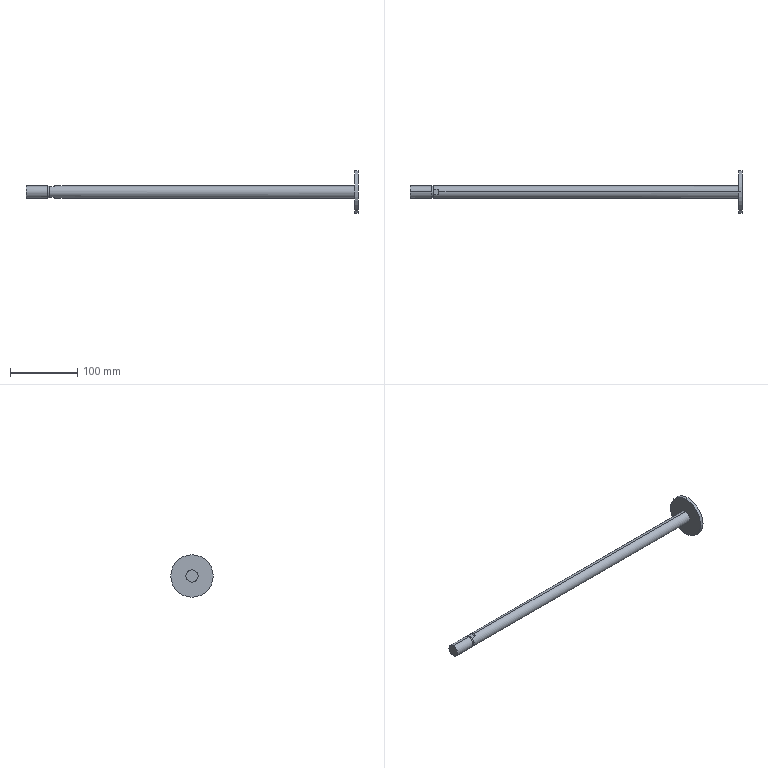Part | STEP file | _JMDBB63-400_ROD | 1 solid | 20 faces | box 492.5 x 63 x 63 mm | volume 139467 mm3 | plane 12 | cylinder 8 | commonest cylinder face diameters 18 x4 16.9 x2 63 x2
STEP:
#1=CARTESIAN_POINT('',(-16.,-2.721,-8.));
#2=VERTEX_POINT('',#1);
#3=CARTESIAN_POINT('',(-16.45,0.,-8.45));
#4=VERTEX_POINT('',#3);
#5=CARTESIAN_POINT('',(-16.,-2.721,-8.));
#6=CARTESIAN_POINT('',(-16.177,-2.201,-8.177));
#7=CARTESIAN_POINT('',(-16.313,-1.663,-8.313));
#8=CARTESIAN_POINT('',(-16.404,-1.113,-8.404));
#9=CARTESIAN_POINT('',(-16.45,-0.5564,-8.45));
#10=CARTESIAN_POINT('',(-16.45,0.,-8.45));
#11=B_SPLINE_CURVE_WITH_KNOTS('',5,(#5,#6,#7,#8,#9,#10),.UNSPECIFIED.,.F.,.U.,(6,6),(0.,5.566),.UNSPECIFIED.);
#12=EDGE_CURVE('',#2,#4,#11,.T.);
#13=ORIENTED_EDGE('',*,*,#12,.T.);
#14=CARTESIAN_POINT('',(-16.,2.721,-8.));
#15=VERTEX_POINT('',#14);
#16=CARTESIAN_POINT('',(-16.45,0.,-8.45));
#17=CARTESIAN_POINT('',(-16.45,0.2882,-8.45));
#18=CARTESIAN_POINT('',(-16.438,0.5763,-8.438));
#19=CARTESIAN_POINT('',(-16.413,0.8637,-8.413));
#20=CARTESIAN_POINT('',(-16.342,1.415,-8.342));
#21=CARTESIAN_POINT('',(-16.227,1.957,-8.227));
#22=CARTESIAN_POINT('',(-16.161,2.215,-8.161));
#23=CARTESIAN_POINT('',(-16.085,2.47,-8.085));
#24=CARTESIAN_POINT('',(-16.,2.721,-8.));
#25=B_SPLINE_CURVE_WITH_KNOTS('',5,(#16,#17,#18,#19,#20,#21,#22,#23,#24),.UNSPECIFIED.,.F.,.U.,(6,3,6),(5.566,8.448,11.129),.UNSPECIFIED.);
#26=EDGE_CURVE('',#4,#15,#25,.T.);
#27=ORIENTED_EDGE('',*,*,#26,.T.);
#28=CARTESIAN_POINT('',(-16.,0.,-8.));
#29=DIRECTION('',(0.,-1.,0.));
#30=VECTOR('',#29,1.);
#31=LINE('',#28,#30);
#32=EDGE_CURVE('',#15,#2,#31,.T.);
#33=ORIENTED_EDGE('',*,*,#32,.T.);
#34=EDGE_LOOP('',(#13,#27,#33));
#35=FACE_OUTER_BOUND('',#34,.T.);
#36=CARTESIAN_POINT('',(-21.,18.,-13.));
#37=DIRECTION('',(0.7071,0.,-0.7071));
#38=DIRECTION('',(-0.7071,0.,-0.7071));
#39=AXIS2_PLACEMENT_3D('',#36,#37,#38);
#40=PLANE('',#39);
#41=ADVANCED_FACE('',(#35),#40,.T.);
#42=CARTESIAN_POINT('',(-16.45,0.,8.45));
#43=VERTEX_POINT('',#42);
#44=CARTESIAN_POINT('',(-19.,0.,8.45));
#45=VERTEX_POINT('',#44);
#46=CARTESIAN_POINT('',(441.5,0.,8.45));
#47=DIRECTION('',(-1.,0.,0.));
#48=VECTOR('',#47,1.);
#49=LINE('',#46,#48);
#50=EDGE_CURVE('',#43,#45,#49,.T.);
#51=ORIENTED_EDGE('',*,*,#50,.T.);
#52=CARTESIAN_POINT('',(-19.,-8.45,0.));
#53=VERTEX_POINT('',#52);
#54=CARTESIAN_POINT('',(-19.,0.,0.));
#55=DIRECTION('',(-1.,0.,0.));
#56=AXIS2_PLACEMENT_3D('',#54,#55,$);
#57=CIRCLE('',#56,8.45);
#58=EDGE_CURVE('',#45,#53,#57,.F.);
#59=ORIENTED_EDGE('',*,*,#58,.T.);
#60=CARTESIAN_POINT('',(-19.,0.,-8.45));
#61=VERTEX_POINT('',#60);
#62=CARTESIAN_POINT('',(-19.,0.,0.));
#63=DIRECTION('',(-1.,0.,0.));
#64=AXIS2_PLACEMENT_3D('',#62,#63,$);
#65=CIRCLE('',#64,8.45);
#66=EDGE_CURVE('',#53,#61,#65,.F.);
#67=ORIENTED_EDGE('',*,*,#66,.T.);
#68=CARTESIAN_POINT('',(441.5,0.,-8.45));
#69=DIRECTION('',(-1.,0.,0.));
#70=VECTOR('',#69,1.);
#71=LINE('',#68,#70);
#72=EDGE_CURVE('',#61,#4,#71,.F.);
#73=ORIENTED_EDGE('',*,*,#72,.T.);
#74=ORIENTED_EDGE('',*,*,#12,.F.);
#75=CARTESIAN_POINT('',(-16.,-2.721,8.));
#76=VERTEX_POINT('',#75);
#77=CARTESIAN_POINT('',(-16.,0.,0.));
#78=DIRECTION('',(-1.,0.,0.));
#79=AXIS2_PLACEMENT_3D('',#77,#78,$);
#80=CIRCLE('',#79,8.45);
#81=EDGE_CURVE('',#76,#2,#80,.F.);
#82=ORIENTED_EDGE('',*,*,#81,.F.);
#83=CARTESIAN_POINT('',(-16.45,0.,8.45));
#84=CARTESIAN_POINT('',(-16.45,-0.9274,8.45));
#85=CARTESIAN_POINT('',(-16.295,-1.854,8.295));
#86=CARTESIAN_POINT('',(-16.,-2.721,8.));
#87=B_SPLINE_CURVE_WITH_KNOTS('',3,(#83,#84,#85,#86),.UNSPECIFIED.,.F.,.U.,(4,4),(0.,5.565),.UNSPECIFIED.);
#88=EDGE_CURVE('',#43,#76,#87,.T.);
#89=ORIENTED_EDGE('',*,*,#88,.F.);
#90=EDGE_LOOP('',(#51,#59,#67,#73,#74,#82,#89));
#91=FACE_OUTER_BOUND('',#90,.T.);
#92=CARTESIAN_POINT('',(441.5,0.,0.));
#93=DIRECTION('',(-1.,0.,0.));
#94=DIRECTION('',(0.,0.,-1.));
#95=AXIS2_PLACEMENT_3D('',#92,#93,#94);
#96=CYLINDRICAL_SURFACE('',#95,8.45);
#97=ADVANCED_FACE('',(#91),#96,.T.);
#98=ORIENTED_EDGE('',*,*,#72,.F.);
#99=CARTESIAN_POINT('',(-19.,8.45,0.));
#100=VERTEX_POINT('',#99);
#101=CARTESIAN_POINT('',(-19.,0.,0.));
#102=DIRECTION('',(-1.,0.,0.));
#103=AXIS2_PLACEMENT_3D('',#101,#102,$);
#104=CIRCLE('',#103,8.45);
#105=EDGE_CURVE('',#61,#100,#104,.F.);
#106=ORIENTED_EDGE('',*,*,#105,.T.);
#107=CARTESIAN_POINT('',(-19.,0.,0.));
#108=DIRECTION('',(-1.,0.,0.));
#109=AXIS2_PLACEMENT_3D('',#107,#108,$);
#110=CIRCLE('',#109,8.45);
#111=EDGE_CURVE('',#100,#45,#110,.F.);
#112=ORIENTED_EDGE('',*,*,#111,.T.);
#113=ORIENTED_EDGE('',*,*,#50,.F.);
#114=CARTESIAN_POINT('',(-16.,2.721,8.));
#115=VERTEX_POINT('',#114);
#116=CARTESIAN_POINT('',(-16.,2.721,8.));
#117=CARTESIAN_POINT('',(-16.295,1.854,8.295));
#118=CARTESIAN_POINT('',(-16.45,0.9274,8.45));
#119=CARTESIAN_POINT('',(-16.45,0.,8.45));
#120=B_SPLINE_CURVE_WITH_KNOTS('',3,(#116,#117,#118,#119),.UNSPECIFIED.,.F.,.U.,(4,4),(0.,5.565),.UNSPECIFIED.);
#121=EDGE_CURVE('',#115,#43,#120,.T.);
#122=ORIENTED_EDGE('',*,*,#121,.F.);
#123=CARTESIAN_POINT('',(-16.,0.,0.));
#124=DIRECTION('',(-1.,0.,0.));
#125=AXIS2_PLACEMENT_3D('',#123,#124,$);
#126=CIRCLE('',#125,8.45);
#127=EDGE_CURVE('',#15,#115,#126,.F.);
#128=ORIENTED_EDGE('',*,*,#127,.F.);
#129=ORIENTED_EDGE('',*,*,#26,.F.);
#130=EDGE_LOOP('',(#98,#106,#112,#113,#122,#128,#129));
#131=FACE_OUTER_BOUND('',#130,.T.);
#132=CARTESIAN_POINT('',(441.5,0.,0.));
#133=DIRECTION('',(-1.,0.,0.));
#134=DIRECTION('',(0.,0.,1.));
#135=AXIS2_PLACEMENT_3D('',#132,#133,#134);
#136=CYLINDRICAL_SURFACE('',#135,8.45);
#137=ADVANCED_FACE('',(#131),#136,.T.);
#138=CARTESIAN_POINT('',(-16.,4.123,-8.));
#139=VERTEX_POINT('',#138);
#140=CARTESIAN_POINT('',(-9.,4.123,-8.));
#141=VERTEX_POINT('',#140);
#142=CARTESIAN_POINT('',(-12.5,4.123,-8.));
#143=DIRECTION('',(1.,0.,0.));
#144=VECTOR('',#143,1.);
#145=LINE('',#142,#144);
#146=EDGE_CURVE('',#139,#141,#145,.T.);
#147=ORIENTED_EDGE('',*,*,#146,.T.);
#148=CARTESIAN_POINT('',(-9.,-4.123,-8.));
#149=VERTEX_POINT('',#148);
#150=CARTESIAN_POINT('',(-9.,0.,-8.));
#151=DIRECTION('',(0.,-1.,0.));
#152=VECTOR('',#151,1.);
#153=LINE('',#150,#152);
#154=EDGE_CURVE('',#141,#149,#153,.T.);
#155=ORIENTED_EDGE('',*,*,#154,.T.);
#156=CARTESIAN_POINT('',(-16.,-4.123,-8.));
#157=VERTEX_POINT('',#156);
#158=CARTESIAN_POINT('',(-12.5,-4.123,-8.));
#159=DIRECTION('',(1.,0.,0.));
#160=VECTOR('',#159,1.);
#161=LINE('',#158,#160);
#162=EDGE_CURVE('',#149,#157,#161,.F.);
#163=ORIENTED_EDGE('',*,*,#162,.T.);
#164=CARTESIAN_POINT('',(-16.,-3.422,-8.));
#165=DIRECTION('',(0.,-1.,0.));
#166=VECTOR('',#165,1.);
#167=LINE('',#164,#166);
#168=EDGE_CURVE('',#2,#157,#167,.T.);
#169=ORIENTED_EDGE('',*,*,#168,.F.);
#170=ORIENTED_EDGE('',*,*,#32,.F.);
#171=CARTESIAN_POINT('',(-16.,3.422,-8.));
#172=DIRECTION('',(0.,-1.,0.));
#173=VECTOR('',#172,1.);
#174=LINE('',#171,#173);
#175=EDGE_CURVE('',#139,#15,#174,.T.);
#176=ORIENTED_EDGE('',*,*,#175,.F.);
#177=EDGE_LOOP('',(#147,#155,#163,#169,#170,#176));
#178=FACE_OUTER_BOUND('',#177,.T.);
#179=CARTESIAN_POINT('',(-16.,18.,-8.));
#180=DIRECTION('',(0.,0.,-1.));
#181=DIRECTION('',(-1.,0.,0.));
#182=AXIS2_PLACEMENT_3D('',#179,#180,#181);
#183=PLANE('',#182);
#184=ADVANCED_FACE('',(#178),#183,.T.);
#185=CARTESIAN_POINT('',(-19.,9.,0.));
#186=VERTEX_POINT('',#185);
#187=CARTESIAN_POINT('',(-19.,0.,9.));
#188=VERTEX_POINT('',#187);
#189=CARTESIAN_POINT('',(-19.,9.,0.));
#190=CARTESIAN_POINT('',(-19.,9.,0.8818));
#191=CARTESIAN_POINT('',(-19.,8.892,1.764));
#192=CARTESIAN_POINT('',(-19.,8.676,2.628));
#193=CARTESIAN_POINT('',(-19.,8.037,4.286));
#194=CARTESIAN_POINT('',(-19.,7.016,5.74));
#195=CARTESIAN_POINT('',(-19.,6.419,6.401));
#196=CARTESIAN_POINT('',(-19.,5.075,7.563));
#197=CARTESIAN_POINT('',(-19.,3.49,8.366));
#198=CARTESIAN_POINT('',(-19.,2.652,8.669));
#199=CARTESIAN_POINT('',(-19.,1.607,8.906));
#200=CARTESIAN_POINT('',(-19.,0.5458,8.986));
#201=CARTESIAN_POINT('',(-19.,0.364,8.995));
#202=CARTESIAN_POINT('',(-19.,0.182,9.));
#203=CARTESIAN_POINT('',(-19.,0.,9.));
#204=B_SPLINE_CURVE_WITH_KNOTS('',5,(#189,#190,#191,#192,#193,#194,#195,#196,#197,#198,#199,#200,#201,#202,#203),.UNSPECIFIED.,.F.,.U.,(6,3,3,3,6),(0.,6.235,12.471,18.706,19.993),.UNSPECIFIED.);
#205=EDGE_CURVE('',#186,#188,#204,.T.);
#206=ORIENTED_EDGE('',*,*,#205,.T.);
#207=CARTESIAN_POINT('',(-19.,-9.,0.));
#208=VERTEX_POINT('',#207);
#209=CARTESIAN_POINT('',(-19.,0.,9.));
#210=CARTESIAN_POINT('',(-19.,-0.6998,9.));
#211=CARTESIAN_POINT('',(-19.,-1.4,8.932));
#212=CARTESIAN_POINT('',(-19.,-2.091,8.796));
#213=CARTESIAN_POINT('',(-19.,-3.613,8.339));
#214=CARTESIAN_POINT('',(-19.,-5.003,7.56));
#215=CARTESIAN_POINT('',(-19.,-5.721,7.032));
#216=CARTESIAN_POINT('',(-19.,-7.012,5.812));
#217=CARTESIAN_POINT('',(-19.,-7.971,4.317));
#218=CARTESIAN_POINT('',(-19.,-8.357,3.513));
#219=CARTESIAN_POINT('',(-19.,-8.756,2.324));
#220=CARTESIAN_POINT('',(-19.,-8.945,1.091));
#221=CARTESIAN_POINT('',(-19.,-8.982,0.7273));
#222=CARTESIAN_POINT('',(-19.,-9.,0.3637));
#223=CARTESIAN_POINT('',(-19.,-9.,0.));
#224=B_SPLINE_CURVE_WITH_KNOTS('',5,(#209,#210,#211,#212,#213,#214,#215,#216,#217,#218,#219,#220,#221,#222,#223),.UNSPECIFIED.,.F.,.U.,(6,3,3,3,6),(19.993,24.941,31.177,37.412,39.983),.UNSPECIFIED.);
#225=EDGE_CURVE('',#188,#208,#224,.T.);
#226=ORIENTED_EDGE('',*,*,#225,.T.);
#227=CARTESIAN_POINT('',(-19.,0.,-9.));
#228=VERTEX_POINT('',#227);
#229=CARTESIAN_POINT('',(-19.,-9.,0.));
#230=CARTESIAN_POINT('',(-19.,-9.,-0.8818));
#231=CARTESIAN_POINT('',(-19.,-8.892,-1.764));
#232=CARTESIAN_POINT('',(-19.,-8.676,-2.628));
#233=CARTESIAN_POINT('',(-19.,-8.037,-4.286));
#234=CARTESIAN_POINT('',(-19.,-7.016,-5.74));
#235=CARTESIAN_POINT('',(-19.,-6.419,-6.401));
#236=CARTESIAN_POINT('',(-19.,-5.075,-7.563));
#237=CARTESIAN_POINT('',(-19.,-3.49,-8.366));
#238=CARTESIAN_POINT('',(-19.,-2.652,-8.669));
#239=CARTESIAN_POINT('',(-19.,-1.607,-8.906));
#240=CARTESIAN_POINT('',(-19.,-0.5458,-8.986));
#241=CARTESIAN_POINT('',(-19.,-0.364,-8.995));
#242=CARTESIAN_POINT('',(-19.,-0.182,-9.));
#243=CARTESIAN_POINT('',(-19.,0.,-9.));
#244=B_SPLINE_CURVE_WITH_KNOTS('',5,(#229,#230,#231,#232,#233,#234,#235,#236,#237,#238,#239,#240,#241,#242,#243),.UNSPECIFIED.,.F.,.U.,(6,3,3,3,6),(0.,6.235,12.471,18.706,19.993),.UNSPECIFIED.);
#245=EDGE_CURVE('',#208,#228,#244,.T.);
#246=ORIENTED_EDGE('',*,*,#245,.T.);
#247=CARTESIAN_POINT('',(-19.,0.,-9.));
#248=CARTESIAN_POINT('',(-19.,0.6998,-9.));
#249=CARTESIAN_POINT('',(-19.,1.4,-8.932));
#250=CARTESIAN_POINT('',(-19.,2.091,-8.796));
#251=CARTESIAN_POINT('',(-19.,3.613,-8.339));
#252=CARTESIAN_POINT('',(-19.,5.003,-7.56));
#253=CARTESIAN_POINT('',(-19.,5.721,-7.032));
#254=CARTESIAN_POINT('',(-19.,7.012,-5.812));
#255=CARTESIAN_POINT('',(-19.,7.971,-4.317));
#256=CARTESIAN_POINT('',(-19.,8.357,-3.513));
#257=CARTESIAN_POINT('',(-19.,8.756,-2.324));
#258=CARTESIAN_POINT('',(-19.,8.945,-1.091));
#259=CARTESIAN_POINT('',(-19.,8.982,-0.7273));
#260=CARTESIAN_POINT('',(-19.,9.,-0.3637));
#261=CARTESIAN_POINT('',(-19.,9.,0.));
#262=B_SPLINE_CURVE_WITH_KNOTS('',5,(#247,#248,#249,#250,#251,#252,#253,#254,#255,#256,#257,#258,#259,#260,#261),.UNSPECIFIED.,.F.,.U.,(6,3,3,3,6),(19.993,24.941,31.177,37.412,39.983),.UNSPECIFIED.);
#263=EDGE_CURVE('',#228,#186,#262,.T.);
#264=ORIENTED_EDGE('',*,*,#263,.T.);
#265=EDGE_LOOP('',(#206,#226,#246,#264));
#266=FACE_OUTER_BOUND('',#265,.T.);
#267=ORIENTED_EDGE('',*,*,#105,.F.);
#268=ORIENTED_EDGE('',*,*,#66,.F.);
#269=ORIENTED_EDGE('',*,*,#58,.F.);
#270=ORIENTED_EDGE('',*,*,#111,.F.);
#271=EDGE_LOOP('',(#267,#268,#269,#270));
#272=FACE_BOUND('',#271,.T.);
#273=CARTESIAN_POINT('',(-19.,9.,0.));
#274=DIRECTION('',(-1.,0.,0.));
#275=DIRECTION('',(0.,0.,1.));
#276=AXIS2_PLACEMENT_3D('',#273,#274,#275);
#277=PLANE('',#276);
#278=ADVANCED_FACE('',(#266,#272),#277,.F.);
#279=ORIENTED_EDGE('',*,*,#168,.T.);
#280=CARTESIAN_POINT('',(-16.,-4.123,8.));
#281=VERTEX_POINT('',#280);
#282=CARTESIAN_POINT('',(-16.,0.000000002,0.));
#283=DIRECTION('',(1.,0.,0.));
#284=AXIS2_PLACEMENT_3D('',#282,#283,$);
#285=CIRCLE('',#284,9.);
#286=EDGE_CURVE('',#281,#157,#285,.T.);
#287=ORIENTED_EDGE('',*,*,#286,.F.);
#288=CARTESIAN_POINT('',(-16.,-3.422,8.));
#289=DIRECTION('',(0.,-1.,0.));
#290=VECTOR('',#289,1.);
#291=LINE('',#288,#290);
#292=EDGE_CURVE('',#76,#281,#291,.T.);
#293=ORIENTED_EDGE('',*,*,#292,.F.);
#294=ORIENTED_EDGE('',*,*,#81,.T.);
#295=EDGE_LOOP('',(#279,#287,#293,#294));
#296=FACE_OUTER_BOUND('',#295,.T.);
#297=CARTESIAN_POINT('',(-16.,8.45,0.));
#298=DIRECTION('',(1.,0.,0.));
#299=DIRECTION('',(0.,0.,-1.));
#300=AXIS2_PLACEMENT_3D('',#297,#298,#299);
#301=PLANE('',#300);
#302=ADVANCED_FACE('',(#296),#301,.F.);
#303=ORIENTED_EDGE('',*,*,#121,.T.);
#304=ORIENTED_EDGE('',*,*,#88,.T.);
#305=CARTESIAN_POINT('',(-16.,0.,8.));
#306=DIRECTION('',(0.,-1.,0.));
#307=VECTOR('',#306,1.);
#308=LINE('',#305,#307);
#309=EDGE_CURVE('',#115,#76,#308,.T.);
#310=ORIENTED_EDGE('',*,*,#309,.F.);
#311=EDGE_LOOP('',(#303,#304,#310));
#312=FACE_OUTER_BOUND('',#311,.T.);
#313=CARTESIAN_POINT('',(-16.,18.,8.));
#314=DIRECTION('',(0.7071,0.,0.7071));
#315=DIRECTION('',(0.7071,0.,-0.7071));
#316=AXIS2_PLACEMENT_3D('',#313,#314,#315);
#317=PLANE('',#316);
#318=ADVANCED_FACE('',(#312),#317,.T.);
#319=ORIENTED_EDGE('',*,*,#175,.T.);
#320=ORIENTED_EDGE('',*,*,#127,.T.);
#321=CARTESIAN_POINT('',(-16.,4.123,8.));
#322=VERTEX_POINT('',#321);
#323=CARTESIAN_POINT('',(-16.,3.422,8.));
#324=DIRECTION('',(0.,-1.,0.));
#325=VECTOR('',#324,1.);
#326=LINE('',#323,#325);
#327=EDGE_CURVE('',#322,#115,#326,.T.);
#328=ORIENTED_EDGE('',*,*,#327,.F.);
#329=CARTESIAN_POINT('',(-16.,0.000000002,0.));
#330=DIRECTION('',(1.,0.,0.));
#331=AXIS2_PLACEMENT_3D('',#329,#330,$);
#332=CIRCLE('',#331,9.);
#333=EDGE_CURVE('',#139,#322,#332,.T.);
#334=ORIENTED_EDGE('',*,*,#333,.F.);
#335=EDGE_LOOP('',(#319,#320,#328,#334));
#336=FACE_OUTER_BOUND('',#335,.T.);
#337=CARTESIAN_POINT('',(-16.,8.45,0.));
#338=DIRECTION('',(1.,0.,0.));
#339=DIRECTION('',(0.,0.,-1.));
#340=AXIS2_PLACEMENT_3D('',#337,#338,#339);
#341=PLANE('',#340);
#342=ADVANCED_FACE('',(#336),#341,.F.);
#343=CARTESIAN_POINT('',(-8.,0.,-9.));
#344=VERTEX_POINT('',#343);
#345=CARTESIAN_POINT('',(436.5,0.,-9.));
#346=VERTEX_POINT('',#345);
#347=CARTESIAN_POINT('',(441.5,0.,-9.));
#348=DIRECTION('',(-1.,0.,0.));
#349=VECTOR('',#348,1.);
#350=LINE('',#347,#349);
#351=EDGE_CURVE('',#344,#346,#350,.F.);
#352=ORIENTED_EDGE('',*,*,#351,.F.);
#353=CARTESIAN_POINT('',(-9.,4.123,-8.));
#354=CARTESIAN_POINT('',(-8.518,3.187,-8.482));
#355=CARTESIAN_POINT('',(-8.173,2.161,-8.827));
#356=CARTESIAN_POINT('',(-8.,1.08,-9.));
#357=CARTESIAN_POINT('',(-8.,0.,-9.));
#358=B_SPLINE_CURVE_WITH_KNOTS('',4,(#353,#354,#355,#356,#357),.UNSPECIFIED.,.F.,.U.,(5,5),(0.,8.643),.UNSPECIFIED.);
#359=EDGE_CURVE('',#141,#344,#358,.T.);
#360=ORIENTED_EDGE('',*,*,#359,.F.);
#361=ORIENTED_EDGE('',*,*,#146,.F.);
#362=ORIENTED_EDGE('',*,*,#333,.T.);
#363=CARTESIAN_POINT('',(-9.,4.123,8.));
#364=VERTEX_POINT('',#363);
#365=CARTESIAN_POINT('',(441.5,4.123,8.));
#366=DIRECTION('',(-1.,0.,0.));
#367=VECTOR('',#366,1.);
#368=LINE('',#365,#367);
#369=EDGE_CURVE('',#364,#322,#368,.T.);
#370=ORIENTED_EDGE('',*,*,#369,.F.);
#371=CARTESIAN_POINT('',(-8.,0.,9.));
#372=VERTEX_POINT('',#371);
#373=CARTESIAN_POINT('',(-8.,0.,9.));
#374=CARTESIAN_POINT('',(-8.,1.08,9.));
#375=CARTESIAN_POINT('',(-8.173,2.161,8.827));
#376=CARTESIAN_POINT('',(-8.518,3.187,8.482));
#377=CARTESIAN_POINT('',(-9.,4.123,8.));
#378=B_SPLINE_CURVE_WITH_KNOTS('',4,(#373,#374,#375,#376,#377),.UNSPECIFIED.,.F.,.U.,(5,5),(0.,8.643),.UNSPECIFIED.);
#379=EDGE_CURVE('',#372,#364,#378,.T.);
#380=ORIENTED_EDGE('',*,*,#379,.F.);
#381=CARTESIAN_POINT('',(436.5,0.,9.));
#382=VERTEX_POINT('',#381);
#383=CARTESIAN_POINT('',(441.5,0.,9.));
#384=DIRECTION('',(-1.,0.,0.));
#385=VECTOR('',#384,1.);
#386=LINE('',#383,#385);
#387=EDGE_CURVE('',#382,#372,#386,.T.);
#388=ORIENTED_EDGE('',*,*,#387,.F.);
#389=CARTESIAN_POINT('',(436.5,9.,0.));
#390=VERTEX_POINT('',#389);
#391=CARTESIAN_POINT('',(436.5,0.,0.));
#392=DIRECTION('',(-1.,0.,0.));
#393=AXIS2_PLACEMENT_3D('',#391,#392,$);
#394=CIRCLE('',#393,9.);
#395=EDGE_CURVE('',#390,#382,#394,.F.);
#396=ORIENTED_EDGE('',*,*,#395,.F.);
#397=CARTESIAN_POINT('',(436.5,0.,0.));
#398=DIRECTION('',(-1.,0.,0.));
#399=AXIS2_PLACEMENT_3D('',#397,#398,$);
#400=CIRCLE('',#399,9.);
#401=EDGE_CURVE('',#346,#390,#400,.F.);
#402=ORIENTED_EDGE('',*,*,#401,.F.);
#403=EDGE_LOOP('',(#352,#360,#361,#362,#370,#380,#388,#396,#402));
#404=FACE_OUTER_BOUND('',#403,.T.);
#405=CARTESIAN_POINT('',(441.5,0.,0.));
#406=DIRECTION('',(-1.,0.,0.));
#407=DIRECTION('',(0.,0.,1.));
#408=AXIS2_PLACEMENT_3D('',#405,#406,#407);
#409=CYLINDRICAL_SURFACE('',#408,9.);
#410=ADVANCED_FACE('',(#404),#409,.T.);
#411=ORIENTED_EDGE('',*,*,#359,.T.);
#412=CARTESIAN_POINT('',(-8.,0.,-9.));
#413=CARTESIAN_POINT('',(-8.,-0.02,-9.));
#414=CARTESIAN_POINT('',(-8.,-0.04,-9.));
#415=CARTESIAN_POINT('',(-8.,-0.05999,-9.));
#416=CARTESIAN_POINT('',(-8.007,-0.9243,-8.993));
#417=CARTESIAN_POINT('',(-8.118,-1.787,-8.882));
#418=CARTESIAN_POINT('',(-8.325,-2.609,-8.675));
#419=CARTESIAN_POINT('',(-8.623,-3.392,-8.377));
#420=CARTESIAN_POINT('',(-9.,-4.123,-8.));
#421=B_SPLINE_CURVE_WITH_KNOTS('',5,(#412,#413,#414,#415,#416,#417,#418,#419,#420),.UNSPECIFIED.,.F.,.U.,(6,3,6),(8.644,8.844,17.287),.UNSPECIFIED.);
#422=EDGE_CURVE('',#344,#149,#421,.T.);
#423=ORIENTED_EDGE('',*,*,#422,.T.);
#424=ORIENTED_EDGE('',*,*,#154,.F.);
#425=EDGE_LOOP('',(#411,#423,#424));
#426=FACE_OUTER_BOUND('',#425,.T.);
#427=CARTESIAN_POINT('',(-9.,18.,-8.));
#428=DIRECTION('',(-0.7071,0.,-0.7071));
#429=DIRECTION('',(-0.7071,0.,0.7071));
#430=AXIS2_PLACEMENT_3D('',#427,#428,#429);
#431=PLANE('',#430);
#432=ADVANCED_FACE('',(#426),#431,.T.);
#433=ORIENTED_EDGE('',*,*,#387,.T.);
#434=CARTESIAN_POINT('',(-9.,-4.123,8.));
#435=VERTEX_POINT('',#434);
#436=CARTESIAN_POINT('',(-9.,-4.123,8.));
#437=CARTESIAN_POINT('',(-8.518,-3.187,8.482));
#438=CARTESIAN_POINT('',(-8.173,-2.161,8.827));
#439=CARTESIAN_POINT('',(-8.,-1.08,9.));
#440=CARTESIAN_POINT('',(-8.,0.,9.));
#441=B_SPLINE_CURVE_WITH_KNOTS('',4,(#436,#437,#438,#439,#440),.UNSPECIFIED.,.F.,.U.,(5,5),(0.,8.643),.UNSPECIFIED.);
#442=EDGE_CURVE('',#435,#372,#441,.T.);
#443=ORIENTED_EDGE('',*,*,#442,.F.);
#444=CARTESIAN_POINT('',(441.5,-4.123,8.));
#445=DIRECTION('',(-1.,0.,0.));
#446=VECTOR('',#445,1.);
#447=LINE('',#444,#446);
#448=EDGE_CURVE('',#281,#435,#447,.F.);
#449=ORIENTED_EDGE('',*,*,#448,.F.);
#450=ORIENTED_EDGE('',*,*,#286,.T.);
#451=ORIENTED_EDGE('',*,*,#162,.F.);
#452=ORIENTED_EDGE('',*,*,#422,.F.);
#453=ORIENTED_EDGE('',*,*,#351,.T.);
#454=CARTESIAN_POINT('',(436.5,-9.,0.));
#455=VERTEX_POINT('',#454);
#456=CARTESIAN_POINT('',(436.5,0.,0.));
#457=DIRECTION('',(-1.,0.,0.));
#458=AXIS2_PLACEMENT_3D('',#456,#457,$);
#459=CIRCLE('',#458,9.);
#460=EDGE_CURVE('',#455,#346,#459,.F.);
#461=ORIENTED_EDGE('',*,*,#460,.F.);
#462=CARTESIAN_POINT('',(436.5,0.,0.));
#463=DIRECTION('',(-1.,0.,0.));
#464=AXIS2_PLACEMENT_3D('',#462,#463,$);
#465=CIRCLE('',#464,9.);
#466=EDGE_CURVE('',#382,#455,#465,.F.);
#467=ORIENTED_EDGE('',*,*,#466,.F.);
#468=EDGE_LOOP('',(#433,#443,#449,#450,#451,#452,#453,#461,#467));
#469=FACE_OUTER_BOUND('',#468,.T.);
#470=CARTESIAN_POINT('',(441.5,0.,0.));
#471=DIRECTION('',(-1.,0.,0.));
#472=DIRECTION('',(0.,0.,-1.));
#473=AXIS2_PLACEMENT_3D('',#470,#471,#472);
#474=CYLINDRICAL_SURFACE('',#473,9.);
#475=ADVANCED_FACE('',(#469),#474,.T.);
#476=CARTESIAN_POINT('',(-51.,0.,-9.));
#477=VERTEX_POINT('',#476);
#478=CARTESIAN_POINT('',(441.5,0.,-9.));
#479=DIRECTION('',(-1.,0.,0.));
#480=VECTOR('',#479,1.);
#481=LINE('',#478,#480);
#482=EDGE_CURVE('',#477,#228,#481,.F.);
#483=ORIENTED_EDGE('',*,*,#482,.F.);
#484=CARTESIAN_POINT('',(-51.,9.,0.));
#485=VERTEX_POINT('',#484);
#486=CARTESIAN_POINT('',(-51.,0.,0.));
#487=DIRECTION('',(-1.,0.,0.));
#488=AXIS2_PLACEMENT_3D('',#486,#487,$);
#489=CIRCLE('',#488,9.);
#490=EDGE_CURVE('',#477,#485,#489,.F.);
#491=ORIENTED_EDGE('',*,*,#490,.T.);
#492=CARTESIAN_POINT('',(-51.,0.,9.));
#493=VERTEX_POINT('',#492);
#494=CARTESIAN_POINT('',(-51.,0.,0.));
#495=DIRECTION('',(-1.,0.,0.));
#496=AXIS2_PLACEMENT_3D('',#494,#495,$);
#497=CIRCLE('',#496,9.);
#498=EDGE_CURVE('',#485,#493,#497,.F.);
#499=ORIENTED_EDGE('',*,*,#498,.T.);
#500=CARTESIAN_POINT('',(441.5,0.,9.));
#501=DIRECTION('',(-1.,0.,0.));
#502=VECTOR('',#501,1.);
#503=LINE('',#500,#502);
#504=EDGE_CURVE('',#188,#493,#503,.T.);
#505=ORIENTED_EDGE('',*,*,#504,.F.);
#506=ORIENTED_EDGE('',*,*,#205,.F.);
#507=ORIENTED_EDGE('',*,*,#263,.F.);
#508=EDGE_LOOP('',(#483,#491,#499,#505,#506,#507));
#509=FACE_OUTER_BOUND('',#508,.T.);
#510=CARTESIAN_POINT('',(441.5,0.,0.));
#511=DIRECTION('',(-1.,0.,0.));
#512=DIRECTION('',(0.,0.,1.));
#513=AXIS2_PLACEMENT_3D('',#510,#511,#512);
#514=CYLINDRICAL_SURFACE('',#513,9.);
#515=ADVANCED_FACE('',(#509),#514,.T.);
#516=ORIENTED_EDGE('',*,*,#504,.T.);
#517=CARTESIAN_POINT('',(-51.,-9.,0.));
#518=VERTEX_POINT('',#517);
#519=CARTESIAN_POINT('',(-51.,0.,0.));
#520=DIRECTION('',(-1.,0.,0.));
#521=AXIS2_PLACEMENT_3D('',#519,#520,$);
#522=CIRCLE('',#521,9.);
#523=EDGE_CURVE('',#493,#518,#522,.F.);
#524=ORIENTED_EDGE('',*,*,#523,.T.);
#525=CARTESIAN_POINT('',(-51.,0.,0.));
#526=DIRECTION('',(-1.,0.,0.));
#527=AXIS2_PLACEMENT_3D('',#525,#526,$);
#528=CIRCLE('',#527,9.);
#529=EDGE_CURVE('',#518,#477,#528,.F.);
#530=ORIENTED_EDGE('',*,*,#529,.T.);
#531=ORIENTED_EDGE('',*,*,#482,.T.);
#532=ORIENTED_EDGE('',*,*,#245,.F.);
#533=ORIENTED_EDGE('',*,*,#225,.F.);
#534=EDGE_LOOP('',(#516,#524,#530,#531,#532,#533));
#535=FACE_OUTER_BOUND('',#534,.T.);
#536=CARTESIAN_POINT('',(441.5,0.,0.));
#537=DIRECTION('',(-1.,0.,0.));
#538=DIRECTION('',(0.,0.,-1.));
#539=AXIS2_PLACEMENT_3D('',#536,#537,#538);
#540=CYLINDRICAL_SURFACE('',#539,9.);
#541=ADVANCED_FACE('',(#535),#540,.T.);
#542=ORIENTED_EDGE('',*,*,#448,.T.);
#543=CARTESIAN_POINT('',(-9.,0.,8.));
#544=DIRECTION('',(0.,-1.,0.));
#545=VECTOR('',#544,1.);
#546=LINE('',#543,#545);
#547=EDGE_CURVE('',#364,#435,#546,.T.);
#548=ORIENTED_EDGE('',*,*,#547,.F.);
#549=ORIENTED_EDGE('',*,*,#369,.T.);
#550=ORIENTED_EDGE('',*,*,#327,.T.);
#551=ORIENTED_EDGE('',*,*,#309,.T.);
#552=ORIENTED_EDGE('',*,*,#292,.T.);
#553=EDGE_LOOP('',(#542,#548,#549,#550,#551,#552));
#554=FACE_OUTER_BOUND('',#553,.T.);
#555=CARTESIAN_POINT('',(-9.,18.,8.));
#556=DIRECTION('',(0.,0.,1.));
#557=DIRECTION('',(1.,0.,0.));
#558=AXIS2_PLACEMENT_3D('',#555,#556,#557);
#559=PLANE('',#558);
#560=ADVANCED_FACE('',(#554),#559,.T.);
#561=ORIENTED_EDGE('',*,*,#442,.T.);
#562=ORIENTED_EDGE('',*,*,#379,.T.);
#563=ORIENTED_EDGE('',*,*,#547,.T.);
#564=EDGE_LOOP('',(#561,#562,#563));
#565=FACE_OUTER_BOUND('',#564,.T.);
#566=CARTESIAN_POINT('',(-4.,18.,13.));
#567=DIRECTION('',(-0.7071,0.,0.7071));
#568=DIRECTION('',(0.7071,0.,0.7071));
#569=AXIS2_PLACEMENT_3D('',#566,#567,#568);
#570=PLANE('',#569);
#571=ADVANCED_FACE('',(#565),#570,.T.);
#572=CARTESIAN_POINT('',(436.5,0.,-31.5));
#573=VERTEX_POINT('',#572);
#574=CARTESIAN_POINT('',(436.5,31.5,0.));
#575=VERTEX_POINT('',#574);
#576=CARTESIAN_POINT('',(436.5,0.,0.));
#577=DIRECTION('',(1.,0.,0.));
#578=AXIS2_PLACEMENT_3D('',#576,#577,$);
#579=CIRCLE('',#578,31.5);
#580=EDGE_CURVE('',#573,#575,#579,.T.);
#581=ORIENTED_EDGE('',*,*,#580,.F.);
#582=CARTESIAN_POINT('',(436.5,-31.5,0.));
#583=VERTEX_POINT('',#582);
#584=CARTESIAN_POINT('',(436.5,0.,0.));
#585=DIRECTION('',(1.,0.,0.));
#586=AXIS2_PLACEMENT_3D('',#584,#585,$);
#587=CIRCLE('',#586,31.5);
#588=EDGE_CURVE('',#583,#573,#587,.T.);
#589=ORIENTED_EDGE('',*,*,#588,.F.);
#590=CARTESIAN_POINT('',(436.5,0.,31.5));
#591=VERTEX_POINT('',#590);
#592=CARTESIAN_POINT('',(436.5,0.,0.));
#593=DIRECTION('',(1.,0.,0.));
#594=AXIS2_PLACEMENT_3D('',#592,#593,$);
#595=CIRCLE('',#594,31.5);
#596=EDGE_CURVE('',#591,#583,#595,.T.);
#597=ORIENTED_EDGE('',*,*,#596,.F.);
#598=CARTESIAN_POINT('',(436.5,0.,0.));
#599=DIRECTION('',(1.,0.,0.));
#600=AXIS2_PLACEMENT_3D('',#598,#599,$);
#601=CIRCLE('',#600,31.5);
#602=EDGE_CURVE('',#575,#591,#601,.T.);
#603=ORIENTED_EDGE('',*,*,#602,.F.);
#604=EDGE_LOOP('',(#581,#589,#597,#603));
#605=FACE_OUTER_BOUND('',#604,.T.);
#606=ORIENTED_EDGE('',*,*,#395,.T.);
#607=ORIENTED_EDGE('',*,*,#466,.T.);
#608=ORIENTED_EDGE('',*,*,#460,.T.);
#609=ORIENTED_EDGE('',*,*,#401,.T.);
#610=EDGE_LOOP('',(#606,#607,#608,#609));
#611=FACE_BOUND('',#610,.T.);
#612=CARTESIAN_POINT('',(436.5,9.,0.));
#613=DIRECTION('',(1.,0.,0.));
#614=DIRECTION('',(0.,0.,-1.));
#615=AXIS2_PLACEMENT_3D('',#612,#613,#614);
#616=PLANE('',#615);
#617=ADVANCED_FACE('',(#605,#611),#616,.F.);
#618=ORIENTED_EDGE('',*,*,#490,.F.);
#619=ORIENTED_EDGE('',*,*,#529,.F.);
#620=ORIENTED_EDGE('',*,*,#523,.F.);
#621=ORIENTED_EDGE('',*,*,#498,.F.);
#622=EDGE_LOOP('',(#618,#619,#620,#621));
#623=FACE_OUTER_BOUND('',#622,.T.);
#624=CARTESIAN_POINT('',(-51.,0.,0.));
#625=DIRECTION('',(1.,0.,0.));
#626=DIRECTION('',(0.,0.,-1.));
#627=AXIS2_PLACEMENT_3D('',#624,#625,#626);
#628=PLANE('',#627);
#629=ADVANCED_FACE('',(#623),#628,.F.);
#630=CARTESIAN_POINT('',(441.5,0.,-31.5));
#631=VERTEX_POINT('',#630);
#632=CARTESIAN_POINT('',(441.5,0.,-31.5));
#633=DIRECTION('',(-1.,0.,0.));
#634=VECTOR('',#633,1.);
#635=LINE('',#632,#634);
#636=EDGE_CURVE('',#573,#631,#635,.F.);
#637=ORIENTED_EDGE('',*,*,#636,.F.);
#638=ORIENTED_EDGE('',*,*,#580,.T.);
#639=ORIENTED_EDGE('',*,*,#602,.T.);
#640=CARTESIAN_POINT('',(441.5,0.,31.5));
#641=VERTEX_POINT('',#640);
#642=CARTESIAN_POINT('',(441.5,0.,31.5));
#643=DIRECTION('',(-1.,0.,0.));
#644=VECTOR('',#643,1.);
#645=LINE('',#642,#644);
#646=EDGE_CURVE('',#641,#591,#645,.T.);
#647=ORIENTED_EDGE('',*,*,#646,.F.);
#648=CARTESIAN_POINT('',(441.5,31.5,0.));
#649=VERTEX_POINT('',#648);
#650=CARTESIAN_POINT('',(441.5,0.,0.));
#651=DIRECTION('',(-1.,0.,0.));
#652=AXIS2_PLACEMENT_3D('',#650,#651,$);
#653=CIRCLE('',#652,31.5);
#654=EDGE_CURVE('',#649,#641,#653,.F.);
#655=ORIENTED_EDGE('',*,*,#654,.F.);
#656=CARTESIAN_POINT('',(441.5,0.,0.));
#657=DIRECTION('',(-1.,0.,0.));
#658=AXIS2_PLACEMENT_3D('',#656,#657,$);
#659=CIRCLE('',#658,31.5);
#660=EDGE_CURVE('',#631,#649,#659,.F.);
#661=ORIENTED_EDGE('',*,*,#660,.F.);
#662=EDGE_LOOP('',(#637,#638,#639,#647,#655,#661));
#663=FACE_OUTER_BOUND('',#662,.T.);
#664=CARTESIAN_POINT('',(441.5,0.,0.));
#665=DIRECTION('',(-1.,0.,0.));
#666=DIRECTION('',(0.,0.,1.));
#667=AXIS2_PLACEMENT_3D('',#664,#665,#666);
#668=CYLINDRICAL_SURFACE('',#667,31.5);
#669=ADVANCED_FACE('',(#663),#668,.T.);
#670=ORIENTED_EDGE('',*,*,#646,.T.);
#671=ORIENTED_EDGE('',*,*,#596,.T.);
#672=ORIENTED_EDGE('',*,*,#588,.T.);
#673=ORIENTED_EDGE('',*,*,#636,.T.);
#674=CARTESIAN_POINT('',(441.5,-31.5,0.));
#675=VERTEX_POINT('',#674);
#676=CARTESIAN_POINT('',(441.5,0.,0.));
#677=DIRECTION('',(-1.,0.,0.));
#678=AXIS2_PLACEMENT_3D('',#676,#677,$);
#679=CIRCLE('',#678,31.5);
#680=EDGE_CURVE('',#675,#631,#679,.F.);
#681=ORIENTED_EDGE('',*,*,#680,.F.);
#682=CARTESIAN_POINT('',(441.5,0.,0.));
#683=DIRECTION('',(-1.,0.,0.));
#684=AXIS2_PLACEMENT_3D('',#682,#683,$);
#685=CIRCLE('',#684,31.5);
#686=EDGE_CURVE('',#641,#675,#685,.F.);
#687=ORIENTED_EDGE('',*,*,#686,.F.);
#688=EDGE_LOOP('',(#670,#671,#672,#673,#681,#687));
#689=FACE_OUTER_BOUND('',#688,.T.);
#690=CARTESIAN_POINT('',(441.5,0.,0.));
#691=DIRECTION('',(-1.,0.,0.));
#692=DIRECTION('',(0.,0.,-1.));
#693=AXIS2_PLACEMENT_3D('',#690,#691,#692);
#694=CYLINDRICAL_SURFACE('',#693,31.5);
#695=ADVANCED_FACE('',(#689),#694,.T.);
#696=ORIENTED_EDGE('',*,*,#654,.T.);
#697=ORIENTED_EDGE('',*,*,#686,.T.);
#698=ORIENTED_EDGE('',*,*,#680,.T.);
#699=ORIENTED_EDGE('',*,*,#660,.T.);
#700=EDGE_LOOP('',(#696,#697,#698,#699));
#701=FACE_OUTER_BOUND('',#700,.T.);
#702=CARTESIAN_POINT('',(441.5,31.5,0.));
#703=DIRECTION('',(-1.,0.,0.));
#704=DIRECTION('',(0.,0.,1.));
#705=AXIS2_PLACEMENT_3D('',#702,#703,#704);
#706=PLANE('',#705);
#707=ADVANCED_FACE('',(#701),#706,.F.);
#708=CLOSED_SHELL('',(#41,#97,#137,#184,#278,#302,#318,#342,#410,#432,#475,#515,#541,#560,#571,#617,#629,#669,#695,#707));
#709=MANIFOLD_SOLID_BREP('',#708);
#710=(LENGTH_UNIT()NAMED_UNIT(*)SI_UNIT(.MILLI.,.METRE.));
#711=UNCERTAINTY_MEASURE_WITH_UNIT(LENGTH_MEASURE(0.005),#710,'','');
#712=(NAMED_UNIT(*)PLANE_ANGLE_UNIT()SI_UNIT($,.RADIAN.));
#713=(NAMED_UNIT(*)SI_UNIT($,.STERADIAN.)SOLID_ANGLE_UNIT());
#714=(GEOMETRIC_REPRESENTATION_CONTEXT(3)GLOBAL_UNCERTAINTY_ASSIGNED_CONTEXT((#711))GLOBAL_UNIT_ASSIGNED_CONTEXT((#710,#712,#713))REPRESENTATION_CONTEXT('',''));
#715=ADVANCED_BREP_SHAPE_REPRESENTATION('',(#709),#714);